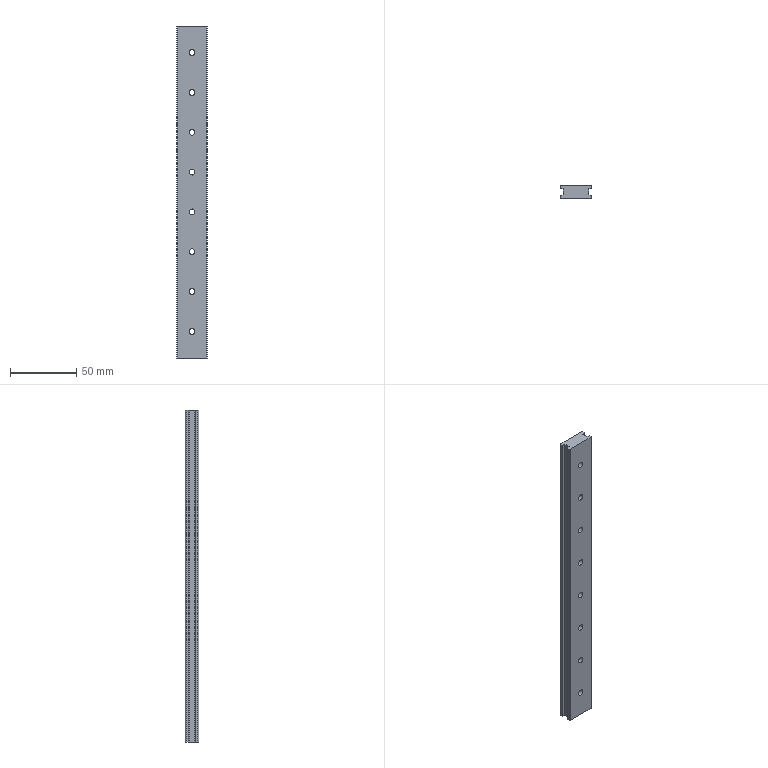Part | STEP file | 1 solid | 42 faces | box 23.2 x 10 x 250 mm | volume 48053 mm3 | plane 26 | cylinder 16 | commonest cylinder face diameters 4.5 x8 10 x8